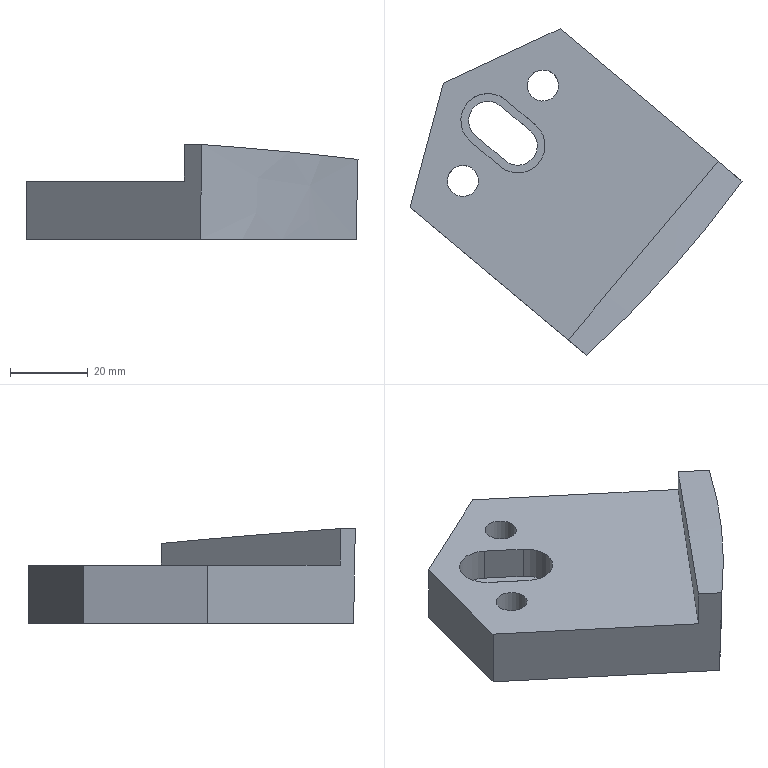Part | NX | features solid 2 | 1 solid | 20 faces | box 85.329 x 83.922 x 24.376 mm | volume 59333 mm3 | plane 12 | cylinder 6 | spline 2 | commonest cylinder face diameters 8 x2 10 x2 14 x2
STEP:
#1=CARTESIAN_POINT('',(-587.956,385.616,-23.5));
#2=VERTEX_POINT('',#1);
#3=CARTESIAN_POINT('',(-587.956,385.616,-30.));
#4=VERTEX_POINT('',#3);
#5=CARTESIAN_POINT('',(-587.956,385.616,-5.));
#6=DIRECTION('',(0.,0.,-1.));
#7=VECTOR('',#6,1000.);
#8=LINE('',#5,#7);
#9=EDGE_CURVE('',#2,#4,#8,.T.);
#10=ORIENTED_EDGE('',*,*,#9,.T.);
#11=CARTESIAN_POINT('',(-594.384,377.956,-30.));
#12=VERTEX_POINT('',#11);
#13=CARTESIAN_POINT('',(-591.17,381.786,-30.));
#14=DIRECTION('',(0.,0.,-1.));
#15=DIRECTION('',(-0.766,0.6428,0.));
#16=AXIS2_PLACEMENT_3D('',#13,#14,#15);
#17=CIRCLE('',#16,5.);
#18=EDGE_CURVE('',#4,#12,#17,.T.);
#19=ORIENTED_EDGE('',*,*,#18,.T.);
#20=CARTESIAN_POINT('',(-594.384,377.956,-23.5));
#21=VERTEX_POINT('',#20);
#22=CARTESIAN_POINT('',(-594.384,377.956,-5.));
#23=DIRECTION('',(0.,0.,-1.));
#24=VECTOR('',#23,1000.);
#25=LINE('',#22,#24);
#26=EDGE_CURVE('',#21,#12,#25,.T.);
#27=ORIENTED_EDGE('',*,*,#26,.F.);
#28=CARTESIAN_POINT('',(-591.17,381.786,-23.5));
#29=DIRECTION('',(0.,0.,-1.));
#30=DIRECTION('',(-0.766,0.6428,0.));
#31=AXIS2_PLACEMENT_3D('',#28,#29,#30);
#32=CIRCLE('',#31,5.);
#33=EDGE_CURVE('',#2,#21,#32,.T.);
#34=ORIENTED_EDGE('',*,*,#33,.F.);
#35=EDGE_LOOP('',(#10,#19,#27,#34));
#36=FACE_BOUND('',#35,.T.);
#37=CARTESIAN_POINT('',(-591.17,381.786,-5.));
#38=DIRECTION('',(0.,0.,-1.));
#39=DIRECTION('',(0.766,-0.6428,0.));
#40=AXIS2_PLACEMENT_3D('',#37,#38,#39);
#41=CYLINDRICAL_SURFACE('',#40,5.);
#42=ADVANCED_FACE('',(#36),#41,.F.);
#43=CARTESIAN_POINT('',(-595.616,392.044,-23.5));
#44=VERTEX_POINT('',#43);
#45=CARTESIAN_POINT('',(-587.956,385.616,-23.5));
#46=DIRECTION('',(-0.766,0.6428,0.));
#47=VECTOR('',#46,1000.);
#48=LINE('',#45,#47);
#49=EDGE_CURVE('',#2,#44,#48,.T.);
#50=ORIENTED_EDGE('',*,*,#49,.T.);
#51=CARTESIAN_POINT('',(-595.616,392.044,-30.));
#52=VERTEX_POINT('',#51);
#53=CARTESIAN_POINT('',(-595.616,392.044,-5.));
#54=DIRECTION('',(0.,0.,-1.));
#55=VECTOR('',#54,1000.);
#56=LINE('',#53,#55);
#57=EDGE_CURVE('',#44,#52,#56,.T.);
#58=ORIENTED_EDGE('',*,*,#57,.T.);
#59=CARTESIAN_POINT('',(-587.956,385.616,-30.));
#60=DIRECTION('',(-0.766,0.6428,0.));
#61=VECTOR('',#60,1000.);
#62=LINE('',#59,#61);
#63=EDGE_CURVE('',#4,#52,#62,.T.);
#64=ORIENTED_EDGE('',*,*,#63,.F.);
#65=ORIENTED_EDGE('',*,*,#9,.F.);
#66=EDGE_LOOP('',(#50,#58,#64,#65));
#67=FACE_BOUND('',#66,.T.);
#68=CARTESIAN_POINT('',(-587.956,385.616,-5.));
#69=DIRECTION('',(0.6428,0.766,0.));
#70=DIRECTION('',(0.,0.,1.));
#71=AXIS2_PLACEMENT_3D('',#68,#69,#70);
#72=PLANE('',#71);
#73=ADVANCED_FACE('',(#67),#72,.F.);
#74=CARTESIAN_POINT('',(-602.044,384.384,-23.5));
#75=VERTEX_POINT('',#74);
#76=CARTESIAN_POINT('',(-602.044,384.384,-30.));
#77=VERTEX_POINT('',#76);
#78=CARTESIAN_POINT('',(-602.044,384.384,-5.));
#79=DIRECTION('',(0.,0.,-1.));
#80=VECTOR('',#79,1000.);
#81=LINE('',#78,#80);
#82=EDGE_CURVE('',#75,#77,#81,.T.);
#83=ORIENTED_EDGE('',*,*,#82,.T.);
#84=CARTESIAN_POINT('',(-598.83,388.214,-30.));
#85=DIRECTION('',(0.,0.,-1.));
#86=DIRECTION('',(-0.766,0.6428,0.));
#87=AXIS2_PLACEMENT_3D('',#84,#85,#86);
#88=CIRCLE('',#87,5.);
#89=EDGE_CURVE('',#77,#52,#88,.T.);
#90=ORIENTED_EDGE('',*,*,#89,.T.);
#91=ORIENTED_EDGE('',*,*,#57,.F.);
#92=CARTESIAN_POINT('',(-598.83,388.214,-23.5));
#93=DIRECTION('',(0.,0.,-1.));
#94=DIRECTION('',(-0.766,0.6428,0.));
#95=AXIS2_PLACEMENT_3D('',#92,#93,#94);
#96=CIRCLE('',#95,5.);
#97=EDGE_CURVE('',#75,#44,#96,.T.);
#98=ORIENTED_EDGE('',*,*,#97,.F.);
#99=EDGE_LOOP('',(#83,#90,#91,#98));
#100=FACE_BOUND('',#99,.T.);
#101=CARTESIAN_POINT('',(-598.83,388.214,-5.));
#102=DIRECTION('',(0.,0.,-1.));
#103=DIRECTION('',(0.766,-0.6428,0.));
#104=AXIS2_PLACEMENT_3D('',#101,#102,#103);
#105=CYLINDRICAL_SURFACE('',#104,5.);
#106=ADVANCED_FACE('',(#100),#105,.F.);
#107=ORIENTED_EDGE('',*,*,#26,.T.);
#108=CARTESIAN_POINT('',(-594.384,377.956,-30.));
#109=DIRECTION('',(-0.766,0.6428,0.));
#110=VECTOR('',#109,1000.);
#111=LINE('',#108,#110);
#112=EDGE_CURVE('',#12,#77,#111,.T.);
#113=ORIENTED_EDGE('',*,*,#112,.T.);
#114=ORIENTED_EDGE('',*,*,#82,.F.);
#115=CARTESIAN_POINT('',(-594.384,377.956,-23.5));
#116=DIRECTION('',(-0.766,0.6428,0.));
#117=VECTOR('',#116,1000.);
#118=LINE('',#115,#117);
#119=EDGE_CURVE('',#21,#75,#118,.T.);
#120=ORIENTED_EDGE('',*,*,#119,.F.);
#121=EDGE_LOOP('',(#107,#113,#114,#120));
#122=FACE_BOUND('',#121,.T.);
#123=CARTESIAN_POINT('',(-594.384,377.956,-5.));
#124=DIRECTION('',(0.6428,0.766,0.));
#125=DIRECTION('',(0.,0.,1.));
#126=AXIS2_PLACEMENT_3D('',#123,#124,#125);
#127=PLANE('',#126);
#128=ADVANCED_FACE('',(#122),#127,.T.);
#129=CARTESIAN_POINT('',(-533.559,372.607,-9.433));
#130=VERTEX_POINT('',#129);
#131=CARTESIAN_POINT('',(-573.65,327.923,-5.624));
#132=VERTEX_POINT('',#131);
#133=CARTESIAN_POINT('',(-573.65,327.923,-5.624));
#134=CARTESIAN_POINT('',(-571.87,329.527,-5.754));
#135=CARTESIAN_POINT('',(-568.31,332.817,-6.02));
#136=CARTESIAN_POINT('',(-563.866,337.139,-6.376));
#137=CARTESIAN_POINT('',(-560.324,340.725,-6.674));
#138=CARTESIAN_POINT('',(-557.672,343.482,-6.904));
#139=CARTESIAN_POINT('',(-555.476,345.828,-7.102));
#140=CARTESIAN_POINT('',(-553.931,347.514,-7.245));
#141=CARTESIAN_POINT('',(-553.07,348.463,-7.325));
#142=CARTESIAN_POINT('',(-552.368,349.243,-7.392));
#143=CARTESIAN_POINT('',(-551.885,349.783,-7.438));
#144=CARTESIAN_POINT('',(-551.157,350.6,-7.507));
#145=CARTESIAN_POINT('',(-549.903,352.021,-7.629));
#146=CARTESIAN_POINT('',(-548.051,354.159,-7.812));
#147=CARTESIAN_POINT('',(-545.771,356.856,-8.045));
#148=CARTESIAN_POINT('',(-542.648,360.647,-8.375));
#149=CARTESIAN_POINT('',(-538.608,365.754,-8.822));
#150=CARTESIAN_POINT('',(-535.256,370.251,-9.222));
#151=CARTESIAN_POINT('',(-533.559,372.607,-9.433));
#152=B_SPLINE_CURVE_WITH_KNOTS('',3,(#133,#134,#135,#136,#137,#138,#139,#140,#141,#142,#143,#144,#145,#146,#147,#148,#149,#150,#151),.UNSPECIFIED.,.F.,.F.,(4,1,1,1,1,1,1,1,1,1,1,1,1,1,1,1,4),(0.,0.125,0.25,0.3125,0.375,0.4375,0.4688,0.4844,0.5,0.5156,0.5312,0.5625,0.625,0.6875,0.75,0.875,1.),.UNSPECIFIED.);
#153=EDGE_CURVE('',#130,#132,#152,.F.);
#154=ORIENTED_EDGE('',*,*,#153,.T.);
#155=CARTESIAN_POINT('',(-574.148,328.341,-30.));
#156=VERTEX_POINT('',#155);
#157=CARTESIAN_POINT('',(-574.148,328.341,-30.));
#158=CARTESIAN_POINT('',(-573.982,328.202,-21.875));
#159=CARTESIAN_POINT('',(-573.816,328.062,-13.749));
#160=CARTESIAN_POINT('',(-573.65,327.923,-5.624));
#161=B_SPLINE_CURVE_WITH_KNOTS('',3,(#157,#158,#159,#160),.UNSPECIFIED.,.F.,.F.,(4,4),(0.,1.),.UNSPECIFIED.);
#162=EDGE_CURVE('',#132,#156,#161,.F.);
#163=ORIENTED_EDGE('',*,*,#162,.T.);
#164=CARTESIAN_POINT('',(-534.064,373.031,-30.));
#165=VERTEX_POINT('',#164);
#166=CARTESIAN_POINT('',(-534.064,373.031,-30.));
#167=CARTESIAN_POINT('',(-545.776,356.775,-30.));
#168=CARTESIAN_POINT('',(-559.138,341.879,-30.));
#169=CARTESIAN_POINT('',(-574.148,328.341,-30.));
#170=B_SPLINE_CURVE_WITH_KNOTS('',3,(#166,#167,#168,#169),.UNSPECIFIED.,.F.,.F.,(4,4),(0.,1.),.UNSPECIFIED.);
#171=EDGE_CURVE('',#156,#165,#170,.F.);
#172=ORIENTED_EDGE('',*,*,#171,.T.);
#173=CARTESIAN_POINT('',(-533.559,372.607,-9.433));
#174=CARTESIAN_POINT('',(-533.727,372.748,-16.288));
#175=CARTESIAN_POINT('',(-533.895,372.889,-23.144));
#176=CARTESIAN_POINT('',(-534.064,373.031,-30.));
#177=B_SPLINE_CURVE_WITH_KNOTS('',3,(#173,#174,#175,#176),.UNSPECIFIED.,.F.,.F.,(4,4),(0.,1.),.UNSPECIFIED.);
#178=EDGE_CURVE('',#130,#165,#177,.T.);
#179=ORIENTED_EDGE('',*,*,#178,.F.);
#180=EDGE_LOOP('',(#154,#163,#172,#179));
#181=FACE_BOUND('',#180,.T.);
#182=CARTESIAN_POINT('',(-573.839,327.669,-3.26));
#183=CARTESIAN_POINT('',(-574.153,327.704,-12.201));
#184=CARTESIAN_POINT('',(-574.467,327.739,-21.141));
#185=CARTESIAN_POINT('',(-574.781,327.775,-30.082));
#186=CARTESIAN_POINT('',(-558.536,341.445,-5.114));
#187=CARTESIAN_POINT('',(-558.875,341.458,-14.064));
#188=CARTESIAN_POINT('',(-559.215,341.47,-23.013));
#189=CARTESIAN_POINT('',(-559.554,341.483,-31.963));
#190=CARTESIAN_POINT('',(-544.913,356.695,-7.155));
#191=CARTESIAN_POINT('',(-545.275,356.683,-16.113));
#192=CARTESIAN_POINT('',(-545.638,356.67,-25.071));
#193=CARTESIAN_POINT('',(-546.,356.658,-34.03));
#194=CARTESIAN_POINT('',(-532.97,373.42,-9.381));
#195=CARTESIAN_POINT('',(-533.353,373.38,-18.348));
#196=CARTESIAN_POINT('',(-533.736,373.339,-27.315));
#197=CARTESIAN_POINT('',(-534.119,373.298,-36.282));
#198=B_SPLINE_SURFACE_WITH_KNOTS('',3,3,((#182,#183,#184,#185),(#186,#187,#188,#189),(#190,#191,#192,#193),(#194,#195,#196,#197)),.UNSPECIFIED.,.F.,.F.,.F.,(4,4),(4,4),(0.4447,0.5603),(2.478,3.15),.UNSPECIFIED.);
#199=ADVANCED_FACE('',(#181),#198,.F.);
#200=CARTESIAN_POINT('',(-578.28,331.808,-5.624));
#201=VERTEX_POINT('',#200);
#202=CARTESIAN_POINT('',(-578.28,331.808,-15.));
#203=VERTEX_POINT('',#202);
#204=CARTESIAN_POINT('',(-578.28,331.808,-5.));
#205=DIRECTION('',(0.,0.,-1.));
#206=VECTOR('',#205,1000.);
#207=LINE('',#204,#206);
#208=EDGE_CURVE('',#201,#203,#207,.T.);
#209=ORIENTED_EDGE('',*,*,#208,.T.);
#210=CARTESIAN_POINT('',(-618.888,365.882,-15.));
#211=VERTEX_POINT('',#210);
#212=CARTESIAN_POINT('',(-572.151,326.665,-15.));
#213=DIRECTION('',(-0.766,0.6428,0.));
#214=VECTOR('',#213,1000.);
#215=LINE('',#212,#214);
#216=EDGE_CURVE('',#203,#211,#215,.T.);
#217=ORIENTED_EDGE('',*,*,#216,.T.);
#218=CARTESIAN_POINT('',(-618.888,365.882,-30.));
#219=VERTEX_POINT('',#218);
#220=CARTESIAN_POINT('',(-618.888,365.882,-5.));
#221=DIRECTION('',(0.,0.,-1.));
#222=VECTOR('',#221,1000.);
#223=LINE('',#220,#222);
#224=EDGE_CURVE('',#211,#219,#223,.T.);
#225=ORIENTED_EDGE('',*,*,#224,.T.);
#226=CARTESIAN_POINT('',(-572.151,326.665,-30.));
#227=DIRECTION('',(-0.766,0.6428,0.));
#228=VECTOR('',#227,1000.);
#229=LINE('',#226,#228);
#230=EDGE_CURVE('',#156,#219,#229,.T.);
#231=ORIENTED_EDGE('',*,*,#230,.F.);
#232=ORIENTED_EDGE('',*,*,#162,.F.);
#233=CARTESIAN_POINT('',(-575.597,329.557,-5.624));
#234=DIRECTION('',(0.766,-0.6428,0.));
#235=VECTOR('',#234,1000.);
#236=LINE('',#233,#235);
#237=EDGE_CURVE('',#201,#132,#236,.T.);
#238=ORIENTED_EDGE('',*,*,#237,.F.);
#239=EDGE_LOOP('',(#209,#217,#225,#231,#232,#238));
#240=FACE_BOUND('',#239,.T.);
#241=CARTESIAN_POINT('',(-572.151,326.665,-5.));
#242=DIRECTION('',(0.6428,0.766,0.));
#243=DIRECTION('',(0.766,-0.6428,0.));
#244=AXIS2_PLACEMENT_3D('',#241,#242,#243);
#245=PLANE('',#244);
#246=ADVANCED_FACE('',(#240),#245,.F.);
#247=CARTESIAN_POINT('',(-610.321,397.856,-15.));
#248=VERTEX_POINT('',#247);
#249=CARTESIAN_POINT('',(-618.888,365.882,-15.));
#250=DIRECTION('',(0.2588,0.9659,0.));
#251=VECTOR('',#250,1000.);
#252=LINE('',#249,#251);
#253=EDGE_CURVE('',#211,#248,#252,.T.);
#254=ORIENTED_EDGE('',*,*,#253,.T.);
#255=CARTESIAN_POINT('',(-610.321,397.856,-30.));
#256=VERTEX_POINT('',#255);
#257=CARTESIAN_POINT('',(-610.321,397.856,-5.));
#258=DIRECTION('',(0.,0.,-1.));
#259=VECTOR('',#258,1000.);
#260=LINE('',#257,#259);
#261=EDGE_CURVE('',#248,#256,#260,.T.);
#262=ORIENTED_EDGE('',*,*,#261,.T.);
#263=CARTESIAN_POINT('',(-618.888,365.882,-30.));
#264=DIRECTION('',(0.2588,0.9659,0.));
#265=VECTOR('',#264,1000.);
#266=LINE('',#263,#265);
#267=EDGE_CURVE('',#219,#256,#266,.T.);
#268=ORIENTED_EDGE('',*,*,#267,.F.);
#269=ORIENTED_EDGE('',*,*,#224,.F.);
#270=EDGE_LOOP('',(#254,#262,#268,#269));
#271=FACE_BOUND('',#270,.T.);
#272=CARTESIAN_POINT('',(-618.888,365.882,-5.));
#273=DIRECTION('',(0.9659,-0.2588,0.));
#274=DIRECTION('',(-0.2588,-0.9659,0.));
#275=AXIS2_PLACEMENT_3D('',#272,#273,#274);
#276=PLANE('',#275);
#277=ADVANCED_FACE('',(#271),#276,.F.);
#278=CARTESIAN_POINT('',(-580.321,411.845,-15.));
#279=VERTEX_POINT('',#278);
#280=CARTESIAN_POINT('',(-580.321,411.845,-30.));
#281=VERTEX_POINT('',#280);
#282=CARTESIAN_POINT('',(-580.321,411.845,-5.));
#283=DIRECTION('',(0.,0.,-1.));
#284=VECTOR('',#283,1000.);
#285=LINE('',#282,#284);
#286=EDGE_CURVE('',#279,#281,#285,.T.);
#287=ORIENTED_EDGE('',*,*,#286,.T.);
#288=CARTESIAN_POINT('',(-580.321,411.845,-30.));
#289=DIRECTION('',(-0.9063,-0.4226,0.));
#290=VECTOR('',#289,1000.);
#291=LINE('',#288,#290);
#292=EDGE_CURVE('',#281,#256,#291,.T.);
#293=ORIENTED_EDGE('',*,*,#292,.T.);
#294=ORIENTED_EDGE('',*,*,#261,.F.);
#295=CARTESIAN_POINT('',(-580.321,411.845,-15.));
#296=DIRECTION('',(-0.9063,-0.4226,0.));
#297=VECTOR('',#296,1000.);
#298=LINE('',#295,#297);
#299=EDGE_CURVE('',#279,#248,#298,.T.);
#300=ORIENTED_EDGE('',*,*,#299,.F.);
#301=EDGE_LOOP('',(#287,#293,#294,#300));
#302=FACE_BOUND('',#301,.T.);
#303=CARTESIAN_POINT('',(-580.321,411.845,-5.));
#304=DIRECTION('',(-0.4226,0.9063,0.));
#305=DIRECTION('',(0.9063,0.4226,0.));
#306=AXIS2_PLACEMENT_3D('',#303,#304,#305);
#307=PLANE('',#306);
#308=ADVANCED_FACE('',(#302),#307,.T.);
#309=CARTESIAN_POINT('',(-587.78,399.828,-15.));
#310=VERTEX_POINT('',#309);
#311=CARTESIAN_POINT('',(-584.715,397.257,-15.));
#312=DIRECTION('',(0.,0.,-1.));
#313=DIRECTION('',(-0.766,0.6428,0.));
#314=AXIS2_PLACEMENT_3D('',#311,#312,#313);
#315=CIRCLE('',#314,4.);
#316=EDGE_CURVE('',#310,#310,#315,.T.);
#317=ORIENTED_EDGE('',*,*,#316,.F.);
#318=EDGE_LOOP('',(#317));
#319=FACE_BOUND('',#318,.T.);
#320=CARTESIAN_POINT('',(-587.78,399.828,-30.));
#321=VERTEX_POINT('',#320);
#322=CARTESIAN_POINT('',(-584.715,397.257,-30.));
#323=DIRECTION('',(0.,0.,-1.));
#324=DIRECTION('',(-0.766,0.6428,0.));
#325=AXIS2_PLACEMENT_3D('',#322,#323,#324);
#326=CIRCLE('',#325,4.);
#327=EDGE_CURVE('',#321,#321,#326,.T.);
#328=ORIENTED_EDGE('',*,*,#327,.T.);
#329=EDGE_LOOP('',(#328));
#330=FACE_BOUND('',#329,.T.);
#331=CARTESIAN_POINT('',(-584.715,397.257,-5.));
#332=DIRECTION('',(0.,0.,-1.));
#333=DIRECTION('',(0.766,-0.6428,0.));
#334=AXIS2_PLACEMENT_3D('',#331,#332,#333);
#335=CYLINDRICAL_SURFACE('',#334,4.);
#336=ADVANCED_FACE('',(#319,#330),#335,.F.);
#337=CARTESIAN_POINT('',(-539.712,377.77,-9.433));
#338=VERTEX_POINT('',#337);
#339=CARTESIAN_POINT('',(-537.03,375.52,-9.433));
#340=DIRECTION('',(0.766,-0.6428,0.));
#341=VECTOR('',#340,1000.);
#342=LINE('',#339,#341);
#343=EDGE_CURVE('',#338,#130,#342,.T.);
#344=ORIENTED_EDGE('',*,*,#343,.T.);
#345=ORIENTED_EDGE('',*,*,#178,.T.);
#346=CARTESIAN_POINT('',(-533.584,372.628,-30.));
#347=DIRECTION('',(-0.766,0.6428,0.));
#348=VECTOR('',#347,1000.);
#349=LINE('',#346,#348);
#350=EDGE_CURVE('',#165,#281,#349,.T.);
#351=ORIENTED_EDGE('',*,*,#350,.T.);
#352=ORIENTED_EDGE('',*,*,#286,.F.);
#353=CARTESIAN_POINT('',(-539.712,377.77,-15.));
#354=VERTEX_POINT('',#353);
#355=CARTESIAN_POINT('',(-533.584,372.628,-15.));
#356=DIRECTION('',(-0.766,0.6428,0.));
#357=VECTOR('',#356,1000.);
#358=LINE('',#355,#357);
#359=EDGE_CURVE('',#354,#279,#358,.T.);
#360=ORIENTED_EDGE('',*,*,#359,.F.);
#361=CARTESIAN_POINT('',(-539.712,377.77,-5.));
#362=DIRECTION('',(0.,0.,-1.));
#363=VECTOR('',#362,1000.);
#364=LINE('',#361,#363);
#365=EDGE_CURVE('',#338,#354,#364,.T.);
#366=ORIENTED_EDGE('',*,*,#365,.F.);
#367=EDGE_LOOP('',(#344,#345,#351,#352,#360,#366));
#368=FACE_BOUND('',#367,.T.);
#369=CARTESIAN_POINT('',(-533.584,372.628,-5.));
#370=DIRECTION('',(0.6428,0.766,0.));
#371=DIRECTION('',(0.766,-0.6428,0.));
#372=AXIS2_PLACEMENT_3D('',#369,#370,#371);
#373=PLANE('',#372);
#374=ADVANCED_FACE('',(#368),#373,.T.);
#375=CARTESIAN_POINT('',(-608.349,375.314,-15.));
#376=VERTEX_POINT('',#375);
#377=CARTESIAN_POINT('',(-605.285,372.743,-15.));
#378=DIRECTION('',(0.,0.,-1.));
#379=DIRECTION('',(-0.766,0.6428,0.));
#380=AXIS2_PLACEMENT_3D('',#377,#378,#379);
#381=CIRCLE('',#380,4.);
#382=EDGE_CURVE('',#376,#376,#381,.F.);
#383=ORIENTED_EDGE('',*,*,#382,.T.);
#384=EDGE_LOOP('',(#383));
#385=FACE_BOUND('',#384,.T.);
#386=CARTESIAN_POINT('',(-608.349,375.314,-30.));
#387=VERTEX_POINT('',#386);
#388=CARTESIAN_POINT('',(-605.285,372.743,-30.));
#389=DIRECTION('',(0.,0.,1.));
#390=DIRECTION('',(-0.766,0.6428,0.));
#391=AXIS2_PLACEMENT_3D('',#388,#389,#390);
#392=CIRCLE('',#391,4.);
#393=EDGE_CURVE('',#387,#387,#392,.T.);
#394=ORIENTED_EDGE('',*,*,#393,.F.);
#395=EDGE_LOOP('',(#394));
#396=FACE_BOUND('',#395,.T.);
#397=CARTESIAN_POINT('',(-605.285,372.743,-5.));
#398=DIRECTION('',(0.,0.,-1.));
#399=DIRECTION('',(0.766,-0.6428,0.));
#400=AXIS2_PLACEMENT_3D('',#397,#398,#399);
#401=CYLINDRICAL_SURFACE('',#400,4.);
#402=ADVANCED_FACE('',(#385,#396),#401,.F.);
#403=ORIENTED_EDGE('',*,*,#18,.F.);
#404=ORIENTED_EDGE('',*,*,#63,.T.);
#405=ORIENTED_EDGE('',*,*,#89,.F.);
#406=ORIENTED_EDGE('',*,*,#112,.F.);
#407=EDGE_LOOP('',(#403,#404,#405,#406));
#408=FACE_BOUND('',#407,.T.);
#409=ORIENTED_EDGE('',*,*,#171,.F.);
#410=ORIENTED_EDGE('',*,*,#230,.T.);
#411=ORIENTED_EDGE('',*,*,#267,.T.);
#412=ORIENTED_EDGE('',*,*,#292,.F.);
#413=ORIENTED_EDGE('',*,*,#350,.F.);
#414=EDGE_LOOP('',(#409,#410,#411,#412,#413));
#415=FACE_BOUND('',#414,.T.);
#416=ORIENTED_EDGE('',*,*,#327,.F.);
#417=EDGE_LOOP('',(#416));
#418=FACE_BOUND('',#417,.T.);
#419=ORIENTED_EDGE('',*,*,#393,.T.);
#420=EDGE_LOOP('',(#419));
#421=FACE_BOUND('',#420,.T.);
#422=CARTESIAN_POINT('',(-533.584,372.628,-30.));
#423=DIRECTION('',(0.,0.,1.));
#424=DIRECTION('',(-0.766,0.6428,0.));
#425=AXIS2_PLACEMENT_3D('',#422,#423,#424);
#426=PLANE('',#425);
#427=ADVANCED_FACE('',(#408,#415,#418,#421),#426,.F.);
#428=CARTESIAN_POINT('',(-586.67,387.148,-15.));
#429=VERTEX_POINT('',#428);
#430=CARTESIAN_POINT('',(-594.331,393.576,-15.));
#431=VERTEX_POINT('',#430);
#432=CARTESIAN_POINT('',(-586.67,387.148,-15.));
#433=DIRECTION('',(-0.766,0.6428,0.));
#434=VECTOR('',#433,1000.);
#435=LINE('',#432,#434);
#436=EDGE_CURVE('',#429,#431,#435,.T.);
#437=ORIENTED_EDGE('',*,*,#436,.T.);
#438=CARTESIAN_POINT('',(-594.331,393.576,-23.5));
#439=VERTEX_POINT('',#438);
#440=CARTESIAN_POINT('',(-594.331,393.576,0.));
#441=DIRECTION('',(0.,0.,-1.));
#442=VECTOR('',#441,1000.);
#443=LINE('',#440,#442);
#444=EDGE_CURVE('',#431,#439,#443,.T.);
#445=ORIENTED_EDGE('',*,*,#444,.T.);
#446=CARTESIAN_POINT('',(-586.67,387.148,-23.5));
#447=VERTEX_POINT('',#446);
#448=CARTESIAN_POINT('',(-586.67,387.148,-23.5));
#449=DIRECTION('',(-0.766,0.6428,0.));
#450=VECTOR('',#449,1000.);
#451=LINE('',#448,#450);
#452=EDGE_CURVE('',#447,#439,#451,.T.);
#453=ORIENTED_EDGE('',*,*,#452,.F.);
#454=CARTESIAN_POINT('',(-586.67,387.148,0.));
#455=DIRECTION('',(0.,0.,-1.));
#456=VECTOR('',#455,1000.);
#457=LINE('',#454,#456);
#458=EDGE_CURVE('',#429,#447,#457,.T.);
#459=ORIENTED_EDGE('',*,*,#458,.F.);
#460=EDGE_LOOP('',(#437,#445,#453,#459));
#461=FACE_BOUND('',#460,.T.);
#462=CARTESIAN_POINT('',(-586.67,387.148,0.));
#463=DIRECTION('',(0.6428,0.766,0.));
#464=DIRECTION('',(0.,0.,1.));
#465=AXIS2_PLACEMENT_3D('',#462,#463,#464);
#466=PLANE('',#465);
#467=ADVANCED_FACE('',(#461),#466,.F.);
#468=CARTESIAN_POINT('',(-603.33,382.852,-15.));
#469=VERTEX_POINT('',#468);
#470=CARTESIAN_POINT('',(-598.83,388.214,-15.));
#471=DIRECTION('',(0.,0.,-1.));
#472=DIRECTION('',(-0.766,0.6428,0.));
#473=AXIS2_PLACEMENT_3D('',#470,#471,#472);
#474=CIRCLE('',#473,7.);
#475=EDGE_CURVE('',#431,#469,#474,.F.);
#476=ORIENTED_EDGE('',*,*,#475,.T.);
#477=CARTESIAN_POINT('',(-603.33,382.852,-23.5));
#478=VERTEX_POINT('',#477);
#479=CARTESIAN_POINT('',(-603.33,382.852,0.));
#480=DIRECTION('',(0.,0.,-1.));
#481=VECTOR('',#480,1000.);
#482=LINE('',#479,#481);
#483=EDGE_CURVE('',#469,#478,#482,.T.);
#484=ORIENTED_EDGE('',*,*,#483,.T.);
#485=CARTESIAN_POINT('',(-598.83,388.214,-23.5));
#486=DIRECTION('',(0.,0.,1.));
#487=DIRECTION('',(-0.766,0.6428,0.));
#488=AXIS2_PLACEMENT_3D('',#485,#486,#487);
#489=CIRCLE('',#488,7.);
#490=EDGE_CURVE('',#439,#478,#489,.T.);
#491=ORIENTED_EDGE('',*,*,#490,.F.);
#492=ORIENTED_EDGE('',*,*,#444,.F.);
#493=EDGE_LOOP('',(#476,#484,#491,#492));
#494=FACE_BOUND('',#493,.T.);
#495=CARTESIAN_POINT('',(-598.83,388.214,0.));
#496=DIRECTION('',(0.,0.,-1.));
#497=DIRECTION('',(0.766,-0.6428,0.));
#498=AXIS2_PLACEMENT_3D('',#495,#496,#497);
#499=CYLINDRICAL_SURFACE('',#498,7.);
#500=ADVANCED_FACE('',(#494),#499,.F.);
#501=CARTESIAN_POINT('',(-595.669,376.424,-15.));
#502=VERTEX_POINT('',#501);
#503=CARTESIAN_POINT('',(-595.669,376.424,-23.5));
#504=VERTEX_POINT('',#503);
#505=CARTESIAN_POINT('',(-595.669,376.424,0.));
#506=DIRECTION('',(0.,0.,-1.));
#507=VECTOR('',#506,1000.);
#508=LINE('',#505,#507);
#509=EDGE_CURVE('',#502,#504,#508,.T.);
#510=ORIENTED_EDGE('',*,*,#509,.T.);
#511=CARTESIAN_POINT('',(-595.669,376.424,-23.5));
#512=DIRECTION('',(-0.766,0.6428,0.));
#513=VECTOR('',#512,1000.);
#514=LINE('',#511,#513);
#515=EDGE_CURVE('',#504,#478,#514,.T.);
#516=ORIENTED_EDGE('',*,*,#515,.T.);
#517=ORIENTED_EDGE('',*,*,#483,.F.);
#518=CARTESIAN_POINT('',(-595.669,376.424,-15.));
#519=DIRECTION('',(-0.766,0.6428,0.));
#520=VECTOR('',#519,1000.);
#521=LINE('',#518,#520);
#522=EDGE_CURVE('',#502,#469,#521,.T.);
#523=ORIENTED_EDGE('',*,*,#522,.F.);
#524=EDGE_LOOP('',(#510,#516,#517,#523));
#525=FACE_BOUND('',#524,.T.);
#526=CARTESIAN_POINT('',(-595.669,376.424,0.));
#527=DIRECTION('',(0.6428,0.766,0.));
#528=DIRECTION('',(0.,0.,1.));
#529=AXIS2_PLACEMENT_3D('',#526,#527,#528);
#530=PLANE('',#529);
#531=ADVANCED_FACE('',(#525),#530,.T.);
#532=ORIENTED_EDGE('',*,*,#458,.T.);
#533=CARTESIAN_POINT('',(-591.17,381.786,-23.5));
#534=DIRECTION('',(0.,0.,-1.));
#535=DIRECTION('',(-0.766,0.6428,0.));
#536=AXIS2_PLACEMENT_3D('',#533,#534,#535);
#537=CIRCLE('',#536,7.);
#538=EDGE_CURVE('',#447,#504,#537,.T.);
#539=ORIENTED_EDGE('',*,*,#538,.T.);
#540=ORIENTED_EDGE('',*,*,#509,.F.);
#541=CARTESIAN_POINT('',(-591.17,381.786,-15.));
#542=DIRECTION('',(0.,0.,-1.));
#543=DIRECTION('',(-0.766,0.6428,0.));
#544=AXIS2_PLACEMENT_3D('',#541,#542,#543);
#545=CIRCLE('',#544,7.);
#546=EDGE_CURVE('',#429,#502,#545,.T.);
#547=ORIENTED_EDGE('',*,*,#546,.F.);
#548=EDGE_LOOP('',(#532,#539,#540,#547));
#549=FACE_BOUND('',#548,.T.);
#550=CARTESIAN_POINT('',(-591.17,381.786,0.));
#551=DIRECTION('',(0.,0.,-1.));
#552=DIRECTION('',(0.766,-0.6428,0.));
#553=AXIS2_PLACEMENT_3D('',#550,#551,#552);
#554=CYLINDRICAL_SURFACE('',#553,7.);
#555=ADVANCED_FACE('',(#549),#554,.F.);
#556=ORIENTED_EDGE('',*,*,#49,.F.);
#557=ORIENTED_EDGE('',*,*,#33,.T.);
#558=ORIENTED_EDGE('',*,*,#119,.T.);
#559=ORIENTED_EDGE('',*,*,#97,.T.);
#560=EDGE_LOOP('',(#556,#557,#558,#559));
#561=FACE_BOUND('',#560,.T.);
#562=ORIENTED_EDGE('',*,*,#452,.T.);
#563=ORIENTED_EDGE('',*,*,#490,.T.);
#564=ORIENTED_EDGE('',*,*,#515,.F.);
#565=ORIENTED_EDGE('',*,*,#538,.F.);
#566=EDGE_LOOP('',(#562,#563,#564,#565));
#567=FACE_BOUND('',#566,.T.);
#568=CARTESIAN_POINT('',(-598.83,388.214,-23.5));
#569=DIRECTION('',(0.,0.,1.));
#570=DIRECTION('',(-0.766,0.6428,0.));
#571=AXIS2_PLACEMENT_3D('',#568,#569,#570);
#572=PLANE('',#571);
#573=ADVANCED_FACE('',(#561,#567),#572,.T.);
#574=CARTESIAN_POINT('',(-578.28,331.808,-5.624));
#575=CARTESIAN_POINT('',(-565.416,347.137,-6.715));
#576=CARTESIAN_POINT('',(-552.56,362.458,-7.977));
#577=CARTESIAN_POINT('',(-539.712,377.77,-9.433));
#578=B_SPLINE_CURVE_WITH_KNOTS('',3,(#574,#575,#576,#577),.UNSPECIFIED.,.F.,.F.,(4,4),(0.,0.06012),.UNSPECIFIED.);
#579=EDGE_CURVE('',#201,#338,#578,.T.);
#580=ORIENTED_EDGE('',*,*,#579,.T.);
#581=ORIENTED_EDGE('',*,*,#365,.T.);
#582=CARTESIAN_POINT('',(-623.275,278.185,-15.));
#583=DIRECTION('',(0.6428,0.766,0.));
#584=VECTOR('',#583,1000.);
#585=LINE('',#582,#584);
#586=EDGE_CURVE('',#203,#354,#585,.T.);
#587=ORIENTED_EDGE('',*,*,#586,.F.);
#588=ORIENTED_EDGE('',*,*,#208,.F.);
#589=EDGE_LOOP('',(#580,#581,#587,#588));
#590=FACE_BOUND('',#589,.T.);
#591=CARTESIAN_POINT('',(-623.275,278.185,-5.));
#592=DIRECTION('',(-0.766,0.6428,0.));
#593=DIRECTION('',(0.,0.,-1.));
#594=AXIS2_PLACEMENT_3D('',#591,#592,#593);
#595=PLANE('',#594);
#596=ADVANCED_FACE('',(#590),#595,.T.);
#597=ORIENTED_EDGE('',*,*,#316,.T.);
#598=EDGE_LOOP('',(#597));
#599=FACE_BOUND('',#598,.T.);
#600=ORIENTED_EDGE('',*,*,#382,.F.);
#601=EDGE_LOOP('',(#600));
#602=FACE_BOUND('',#601,.T.);
#603=ORIENTED_EDGE('',*,*,#546,.T.);
#604=ORIENTED_EDGE('',*,*,#522,.T.);
#605=ORIENTED_EDGE('',*,*,#475,.F.);
#606=ORIENTED_EDGE('',*,*,#436,.F.);
#607=EDGE_LOOP('',(#603,#604,#605,#606));
#608=FACE_BOUND('',#607,.T.);
#609=ORIENTED_EDGE('',*,*,#586,.T.);
#610=ORIENTED_EDGE('',*,*,#359,.T.);
#611=ORIENTED_EDGE('',*,*,#299,.T.);
#612=ORIENTED_EDGE('',*,*,#253,.F.);
#613=ORIENTED_EDGE('',*,*,#216,.F.);
#614=EDGE_LOOP('',(#609,#610,#611,#612,#613));
#615=FACE_BOUND('',#614,.T.);
#616=CARTESIAN_POINT('',(-623.275,278.185,-15.));
#617=DIRECTION('',(0.,0.,1.));
#618=DIRECTION('',(-0.766,0.6428,0.));
#619=AXIS2_PLACEMENT_3D('',#616,#617,#618);
#620=PLANE('',#619);
#621=ADVANCED_FACE('',(#599,#602,#608,#615),#620,.T.);
#622=ORIENTED_EDGE('',*,*,#153,.F.);
#623=ORIENTED_EDGE('',*,*,#343,.F.);
#624=ORIENTED_EDGE('',*,*,#579,.F.);
#625=ORIENTED_EDGE('',*,*,#237,.T.);
#626=EDGE_LOOP('',(#622,#623,#624,#625));
#627=FACE_BOUND('',#626,.T.);
#628=CARTESIAN_POINT('',(-579.695,332.995,-5.624));
#629=CARTESIAN_POINT('',(-572.476,326.938,-5.624));
#630=CARTESIAN_POINT('',(-565.307,346.953,-6.711));
#631=CARTESIAN_POINT('',(-558.088,340.895,-6.711));
#632=CARTESIAN_POINT('',(-552.177,362.206,-7.981));
#633=CARTESIAN_POINT('',(-544.958,356.148,-7.981));
#634=CARTESIAN_POINT('',(-540.735,378.629,-9.433));
#635=CARTESIAN_POINT('',(-533.516,372.571,-9.433));
#636=B_SPLINE_SURFACE_WITH_KNOTS('',3,1,((#628,#629),(#630,#631),(#632,#633),(#634,#635)),.SURF_OF_LINEAR_EXTRUSION.,.F.,.F.,.F.,(4,4),(2,2),(0.05486,0.2386),(0.,1.),.PIECEWISE_BEZIER_KNOTS.);
#637=ADVANCED_FACE('',(#627),#636,.F.);
#638=CLOSED_SHELL('',(#42,#73,#106,#128,#199,#246,#277,#308,#336,#374,#402,#427,#467,#500,#531,#555,#573,#596,#621,#637));
#639=MANIFOLD_SOLID_BREP('',#638);
#640=(LENGTH_UNIT()NAMED_UNIT(*)SI_UNIT(.MILLI.,.METRE.));
#641=UNCERTAINTY_MEASURE_WITH_UNIT(LENGTH_MEASURE(0.0508),#640,'','');
#642=(NAMED_UNIT(*)PLANE_ANGLE_UNIT()SI_UNIT($,.RADIAN.));
#643=(NAMED_UNIT(*)SI_UNIT($,.STERADIAN.)SOLID_ANGLE_UNIT());
#644=(GEOMETRIC_REPRESENTATION_CONTEXT(3)GLOBAL_UNCERTAINTY_ASSIGNED_CONTEXT((#641))GLOBAL_UNIT_ASSIGNED_CONTEXT((#640,#642,#643))REPRESENTATION_CONTEXT('',''));
#645=ADVANCED_BREP_SHAPE_REPRESENTATION('',(#639),#644);